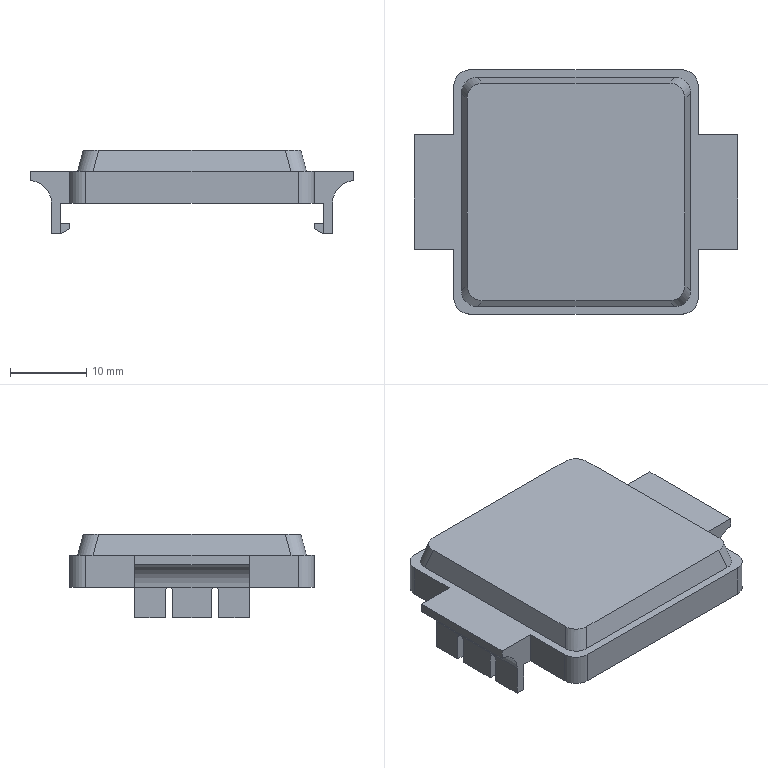Part | SolidWorks | features BaseBody 1 | 1 solid | 81 faces | box 42.4 x 32 x 11 mm | volume 2245 mm3 | plane 57 | cylinder 24 | commonest cylinder face diameters 2.2 x8 4.2 x8 1 x6 6 x2